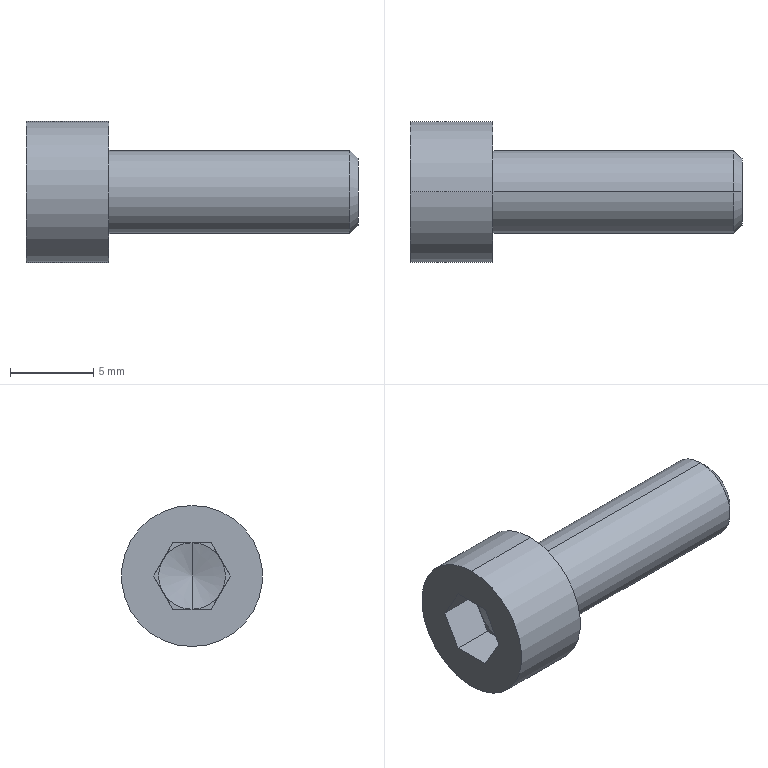Part | STEP file | 11-CB5_15_1-ab11 | 1 solid | 23 faces | box 20 x 8.5 x 8.5 mm | volume 539.598 mm3 | plane 15 | cone 4 | cylinder 4 | commonest cylinder face diameters 5 x2 8.5 x2